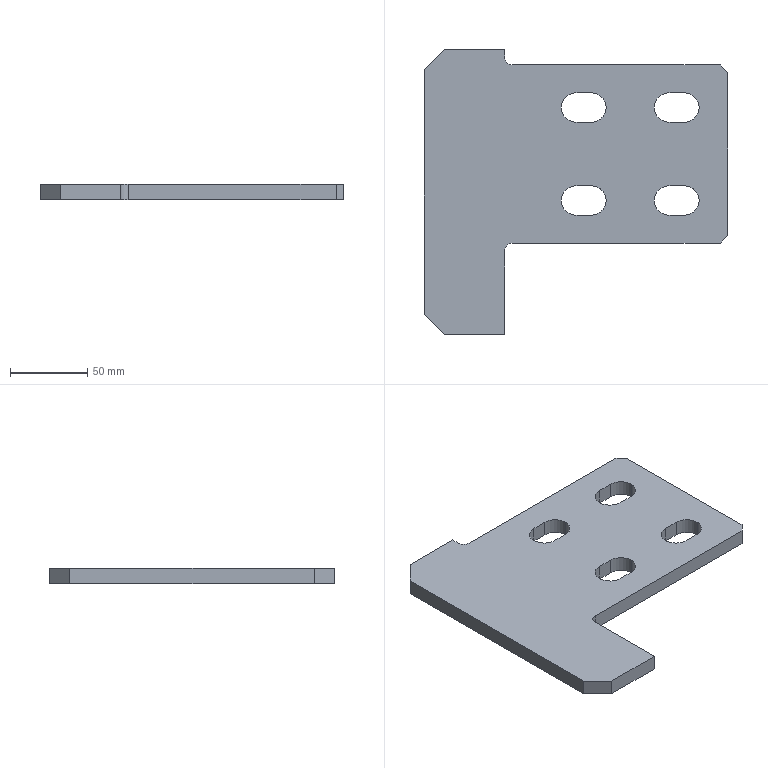Part | STEP file | 筋Plate-200×100-150 -45度 | 1 solid | 36 faces | box 196 x 184 x 10 mm | volume 240506 mm3 | plane 22 | cylinder 14 | commonest cylinder face diameters 19 x12 10 x2